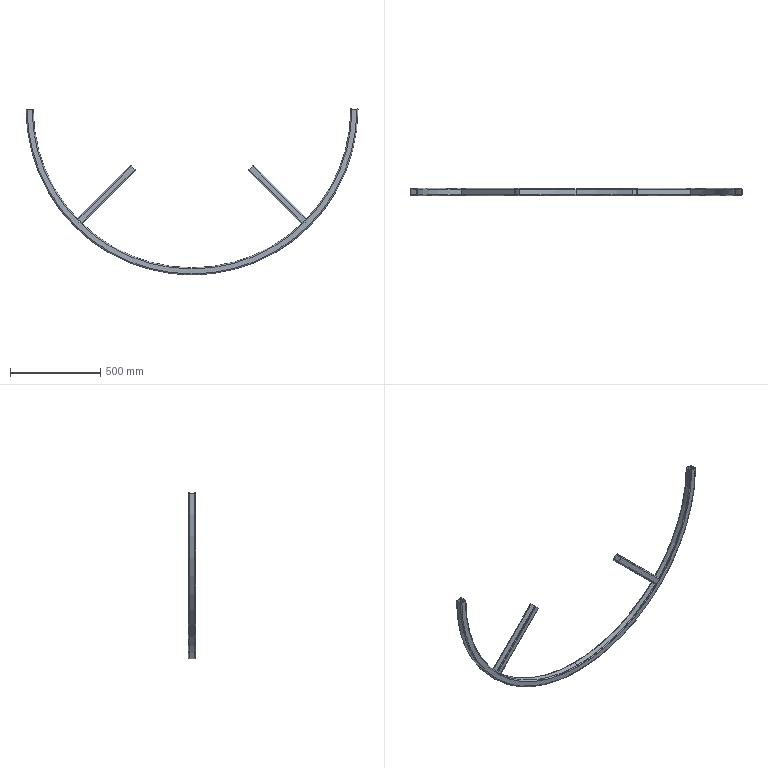Part | SolidWorks | features WeldMemberFeat 1, WeldmentFeature 1 | 3 solids | 66 faces | box 1840 x 40 x 920 mm | volume 1638745 mm3 | cylinder 26 | plane 24 | torus 16 | commonest cylinder face diameters 5.6 x8 12 x8 1760 x4 1766 x2 1834 x2 1840 x2